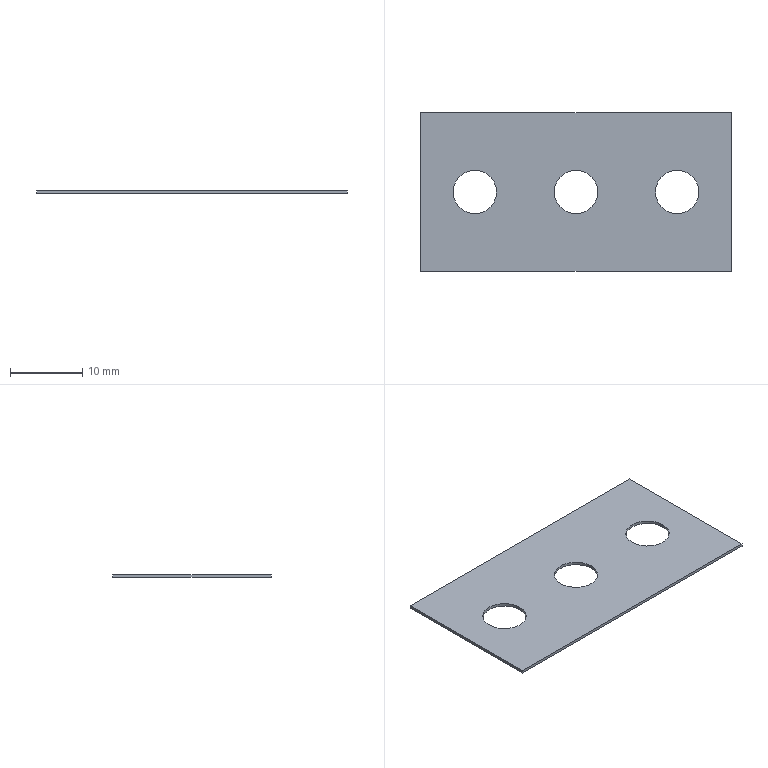Part | SolidWorks | features Extrusion 1, ICE 1 | 1 solid | 12 faces | box 43 x 22 x 0.4 mm | volume 344.471 mm3 | cylinder 6 | plane 6 | commonest cylinder face diameters 6 x6
STEP:
#1=CARTESIAN_POINT('',(11.,0.,0.));
#2=VERTEX_POINT('',#1);
#3=CARTESIAN_POINT('',(17.,0.,0.));
#4=VERTEX_POINT('',#3);
#5=CARTESIAN_POINT('',(14.,0.,0.));
#6=DIRECTION('',(0.,0.,1.));
#7=DIRECTION('',(1.,0.,0.));
#8=AXIS2_PLACEMENT_3D('',#5,#6,#7);
#9=CIRCLE('',#8,3.);
#10=EDGE_CURVE('',#2,#4,#9,.T.);
#11=ORIENTED_EDGE('',*,*,#10,.F.);
#12=CARTESIAN_POINT('',(11.,0.,0.4));
#13=VERTEX_POINT('',#12);
#14=CARTESIAN_POINT('',(11.,0.,0.));
#15=DIRECTION('',(0.,0.,1.));
#16=VECTOR('',#15,1000.);
#17=LINE('',#14,#16);
#18=EDGE_CURVE('',#2,#13,#17,.T.);
#19=ORIENTED_EDGE('',*,*,#18,.T.);
#20=CARTESIAN_POINT('',(17.,0.,0.4));
#21=VERTEX_POINT('',#20);
#22=CARTESIAN_POINT('',(14.,0.,0.4));
#23=DIRECTION('',(0.,0.,1.));
#24=DIRECTION('',(1.,0.,0.));
#25=AXIS2_PLACEMENT_3D('',#22,#23,#24);
#26=CIRCLE('',#25,3.);
#27=EDGE_CURVE('',#13,#21,#26,.T.);
#28=ORIENTED_EDGE('',*,*,#27,.T.);
#29=CARTESIAN_POINT('',(17.,0.,0.));
#30=DIRECTION('',(0.,0.,1.));
#31=VECTOR('',#30,1000.);
#32=LINE('',#29,#31);
#33=EDGE_CURVE('',#4,#21,#32,.T.);
#34=ORIENTED_EDGE('',*,*,#33,.F.);
#35=EDGE_LOOP('',(#11,#19,#28,#34));
#36=FACE_OUTER_BOUND('',#35,.T.);
#37=CARTESIAN_POINT('',(14.,0.,0.));
#38=DIRECTION('',(0.,0.,1.));
#39=DIRECTION('',(1.,0.,0.));
#40=AXIS2_PLACEMENT_3D('',#37,#38,#39);
#41=CYLINDRICAL_SURFACE('',#40,3.);
#42=ADVANCED_FACE('',(#36),#41,.F.);
#43=CARTESIAN_POINT('',(-17.,0.,0.));
#44=VERTEX_POINT('',#43);
#45=CARTESIAN_POINT('',(-11.,0.,0.));
#46=VERTEX_POINT('',#45);
#47=CARTESIAN_POINT('',(-14.,0.,0.));
#48=DIRECTION('',(0.,0.,1.));
#49=DIRECTION('',(1.,0.,0.));
#50=AXIS2_PLACEMENT_3D('',#47,#48,#49);
#51=CIRCLE('',#50,3.);
#52=EDGE_CURVE('',#44,#46,#51,.T.);
#53=ORIENTED_EDGE('',*,*,#52,.F.);
#54=CARTESIAN_POINT('',(-17.,0.,0.4));
#55=VERTEX_POINT('',#54);
#56=CARTESIAN_POINT('',(-17.,0.,0.));
#57=DIRECTION('',(0.,0.,1.));
#58=VECTOR('',#57,1000.);
#59=LINE('',#56,#58);
#60=EDGE_CURVE('',#44,#55,#59,.T.);
#61=ORIENTED_EDGE('',*,*,#60,.T.);
#62=CARTESIAN_POINT('',(-11.,0.,0.4));
#63=VERTEX_POINT('',#62);
#64=CARTESIAN_POINT('',(-14.,0.,0.4));
#65=DIRECTION('',(0.,0.,1.));
#66=DIRECTION('',(1.,0.,0.));
#67=AXIS2_PLACEMENT_3D('',#64,#65,#66);
#68=CIRCLE('',#67,3.);
#69=EDGE_CURVE('',#55,#63,#68,.T.);
#70=ORIENTED_EDGE('',*,*,#69,.T.);
#71=CARTESIAN_POINT('',(-11.,0.,0.));
#72=DIRECTION('',(0.,0.,1.));
#73=VECTOR('',#72,1000.);
#74=LINE('',#71,#73);
#75=EDGE_CURVE('',#46,#63,#74,.T.);
#76=ORIENTED_EDGE('',*,*,#75,.F.);
#77=EDGE_LOOP('',(#53,#61,#70,#76));
#78=FACE_OUTER_BOUND('',#77,.T.);
#79=CARTESIAN_POINT('',(-14.,0.,0.));
#80=DIRECTION('',(0.,0.,1.));
#81=DIRECTION('',(1.,0.,0.));
#82=AXIS2_PLACEMENT_3D('',#79,#80,#81);
#83=CYLINDRICAL_SURFACE('',#82,3.);
#84=ADVANCED_FACE('',(#78),#83,.F.);
#85=CARTESIAN_POINT('',(-3.,0.,0.));
#86=VERTEX_POINT('',#85);
#87=CARTESIAN_POINT('',(3.,0.,0.));
#88=VERTEX_POINT('',#87);
#89=CARTESIAN_POINT('',(0.,0.,0.));
#90=DIRECTION('',(0.,0.,1.));
#91=DIRECTION('',(1.,0.,0.));
#92=AXIS2_PLACEMENT_3D('',#89,#90,#91);
#93=CIRCLE('',#92,3.);
#94=EDGE_CURVE('',#86,#88,#93,.T.);
#95=ORIENTED_EDGE('',*,*,#94,.F.);
#96=CARTESIAN_POINT('',(-3.,0.,0.4));
#97=VERTEX_POINT('',#96);
#98=CARTESIAN_POINT('',(-3.,0.,0.));
#99=DIRECTION('',(0.,0.,1.));
#100=VECTOR('',#99,1000.);
#101=LINE('',#98,#100);
#102=EDGE_CURVE('',#86,#97,#101,.T.);
#103=ORIENTED_EDGE('',*,*,#102,.T.);
#104=CARTESIAN_POINT('',(3.,0.,0.4));
#105=VERTEX_POINT('',#104);
#106=CARTESIAN_POINT('',(0.,0.,0.4));
#107=DIRECTION('',(0.,0.,1.));
#108=DIRECTION('',(1.,0.,0.));
#109=AXIS2_PLACEMENT_3D('',#106,#107,#108);
#110=CIRCLE('',#109,3.);
#111=EDGE_CURVE('',#97,#105,#110,.T.);
#112=ORIENTED_EDGE('',*,*,#111,.T.);
#113=CARTESIAN_POINT('',(3.,0.,0.));
#114=DIRECTION('',(0.,0.,1.));
#115=VECTOR('',#114,1000.);
#116=LINE('',#113,#115);
#117=EDGE_CURVE('',#88,#105,#116,.T.);
#118=ORIENTED_EDGE('',*,*,#117,.F.);
#119=EDGE_LOOP('',(#95,#103,#112,#118));
#120=FACE_OUTER_BOUND('',#119,.T.);
#121=CARTESIAN_POINT('',(0.,0.,0.));
#122=DIRECTION('',(0.,0.,1.));
#123=DIRECTION('',(1.,0.,0.));
#124=AXIS2_PLACEMENT_3D('',#121,#122,#123);
#125=CYLINDRICAL_SURFACE('',#124,3.);
#126=ADVANCED_FACE('',(#120),#125,.F.);
#127=CARTESIAN_POINT('',(21.5,-11.,0.));
#128=VERTEX_POINT('',#127);
#129=CARTESIAN_POINT('',(21.5,11.,0.));
#130=VERTEX_POINT('',#129);
#131=CARTESIAN_POINT('',(21.5,-11.,0.));
#132=DIRECTION('',(0.,1.,0.));
#133=VECTOR('',#132,1000.);
#134=LINE('',#131,#133);
#135=EDGE_CURVE('',#128,#130,#134,.T.);
#136=ORIENTED_EDGE('',*,*,#135,.T.);
#137=CARTESIAN_POINT('',(21.5,11.,0.4));
#138=VERTEX_POINT('',#137);
#139=CARTESIAN_POINT('',(21.5,11.,0.4));
#140=DIRECTION('',(0.,0.,-1.));
#141=VECTOR('',#140,1000.);
#142=LINE('',#139,#141);
#143=EDGE_CURVE('',#138,#130,#142,.T.);
#144=ORIENTED_EDGE('',*,*,#143,.F.);
#145=CARTESIAN_POINT('',(21.5,-11.,0.4));
#146=VERTEX_POINT('',#145);
#147=CARTESIAN_POINT('',(21.5,-11.,0.4));
#148=DIRECTION('',(0.,1.,0.));
#149=VECTOR('',#148,1000.);
#150=LINE('',#147,#149);
#151=EDGE_CURVE('',#146,#138,#150,.T.);
#152=ORIENTED_EDGE('',*,*,#151,.F.);
#153=CARTESIAN_POINT('',(21.5,-11.,0.4));
#154=DIRECTION('',(0.,0.,-1.));
#155=VECTOR('',#154,1000.);
#156=LINE('',#153,#155);
#157=EDGE_CURVE('',#146,#128,#156,.T.);
#158=ORIENTED_EDGE('',*,*,#157,.T.);
#159=EDGE_LOOP('',(#136,#144,#152,#158));
#160=FACE_OUTER_BOUND('',#159,.T.);
#161=CARTESIAN_POINT('',(21.5,-11.,0.4));
#162=DIRECTION('',(-1.,0.,0.));
#163=DIRECTION('',(0.,0.,1.));
#164=AXIS2_PLACEMENT_3D('',#161,#162,#163);
#165=PLANE('',#164);
#166=ADVANCED_FACE('',(#160),#165,.F.);
#167=CARTESIAN_POINT('',(-21.5,11.,0.));
#168=VERTEX_POINT('',#167);
#169=CARTESIAN_POINT('',(-21.5,11.,0.));
#170=DIRECTION('',(-1.,0.,0.));
#171=VECTOR('',#170,1000.);
#172=LINE('',#169,#171);
#173=EDGE_CURVE('',#130,#168,#172,.T.);
#174=ORIENTED_EDGE('',*,*,#173,.T.);
#175=CARTESIAN_POINT('',(-21.5,11.,0.4));
#176=VERTEX_POINT('',#175);
#177=CARTESIAN_POINT('',(-21.5,11.,0.4));
#178=DIRECTION('',(0.,0.,-1.));
#179=VECTOR('',#178,1000.);
#180=LINE('',#177,#179);
#181=EDGE_CURVE('',#176,#168,#180,.T.);
#182=ORIENTED_EDGE('',*,*,#181,.F.);
#183=CARTESIAN_POINT('',(-21.5,11.,0.4));
#184=DIRECTION('',(-1.,0.,0.));
#185=VECTOR('',#184,1000.);
#186=LINE('',#183,#185);
#187=EDGE_CURVE('',#138,#176,#186,.T.);
#188=ORIENTED_EDGE('',*,*,#187,.F.);
#189=ORIENTED_EDGE('',*,*,#143,.T.);
#190=EDGE_LOOP('',(#174,#182,#188,#189));
#191=FACE_OUTER_BOUND('',#190,.T.);
#192=CARTESIAN_POINT('',(-21.5,11.,0.4));
#193=DIRECTION('',(0.,-1.,0.));
#194=DIRECTION('',(0.,0.,-1.));
#195=AXIS2_PLACEMENT_3D('',#192,#193,#194);
#196=PLANE('',#195);
#197=ADVANCED_FACE('',(#191),#196,.F.);
#198=CARTESIAN_POINT('',(-21.5,-11.,0.));
#199=VERTEX_POINT('',#198);
#200=CARTESIAN_POINT('',(-21.5,-11.,0.));
#201=DIRECTION('',(0.,-1.,0.));
#202=VECTOR('',#201,1000.);
#203=LINE('',#200,#202);
#204=EDGE_CURVE('',#168,#199,#203,.T.);
#205=ORIENTED_EDGE('',*,*,#204,.T.);
#206=CARTESIAN_POINT('',(-21.5,-11.,0.4));
#207=VERTEX_POINT('',#206);
#208=CARTESIAN_POINT('',(-21.5,-11.,0.4));
#209=DIRECTION('',(0.,0.,-1.));
#210=VECTOR('',#209,1000.);
#211=LINE('',#208,#210);
#212=EDGE_CURVE('',#207,#199,#211,.T.);
#213=ORIENTED_EDGE('',*,*,#212,.F.);
#214=CARTESIAN_POINT('',(-21.5,-11.,0.4));
#215=DIRECTION('',(0.,-1.,0.));
#216=VECTOR('',#215,1000.);
#217=LINE('',#214,#216);
#218=EDGE_CURVE('',#176,#207,#217,.T.);
#219=ORIENTED_EDGE('',*,*,#218,.F.);
#220=ORIENTED_EDGE('',*,*,#181,.T.);
#221=EDGE_LOOP('',(#205,#213,#219,#220));
#222=FACE_OUTER_BOUND('',#221,.T.);
#223=CARTESIAN_POINT('',(-21.5,-11.,0.4));
#224=DIRECTION('',(1.,0.,0.));
#225=DIRECTION('',(0.,0.,-1.));
#226=AXIS2_PLACEMENT_3D('',#223,#224,#225);
#227=PLANE('',#226);
#228=ADVANCED_FACE('',(#222),#227,.F.);
#229=CARTESIAN_POINT('',(-21.5,-11.,0.));
#230=DIRECTION('',(1.,0.,0.));
#231=VECTOR('',#230,1000.);
#232=LINE('',#229,#231);
#233=EDGE_CURVE('',#199,#128,#232,.T.);
#234=ORIENTED_EDGE('',*,*,#233,.T.);
#235=ORIENTED_EDGE('',*,*,#157,.F.);
#236=CARTESIAN_POINT('',(-21.5,-11.,0.4));
#237=DIRECTION('',(1.,0.,0.));
#238=VECTOR('',#237,1000.);
#239=LINE('',#236,#238);
#240=EDGE_CURVE('',#207,#146,#239,.T.);
#241=ORIENTED_EDGE('',*,*,#240,.F.);
#242=ORIENTED_EDGE('',*,*,#212,.T.);
#243=EDGE_LOOP('',(#234,#235,#241,#242));
#244=FACE_OUTER_BOUND('',#243,.T.);
#245=CARTESIAN_POINT('',(-21.5,-11.,0.4));
#246=DIRECTION('',(0.,1.,0.));
#247=DIRECTION('',(0.,0.,1.));
#248=AXIS2_PLACEMENT_3D('',#245,#246,#247);
#249=PLANE('',#248);
#250=ADVANCED_FACE('',(#244),#249,.F.);
#251=CARTESIAN_POINT('',(14.,0.,0.4));
#252=DIRECTION('',(0.,0.,1.));
#253=DIRECTION('',(1.,0.,0.));
#254=AXIS2_PLACEMENT_3D('',#251,#252,#253);
#255=CIRCLE('',#254,3.);
#256=EDGE_CURVE('',#21,#13,#255,.T.);
#257=ORIENTED_EDGE('',*,*,#256,.F.);
#258=ORIENTED_EDGE('',*,*,#27,.F.);
#259=EDGE_LOOP('',(#257,#258));
#260=FACE_BOUND('',#259,.T.);
#261=CARTESIAN_POINT('',(-14.,0.,0.4));
#262=DIRECTION('',(0.,0.,1.));
#263=DIRECTION('',(1.,0.,0.));
#264=AXIS2_PLACEMENT_3D('',#261,#262,#263);
#265=CIRCLE('',#264,3.);
#266=EDGE_CURVE('',#63,#55,#265,.T.);
#267=ORIENTED_EDGE('',*,*,#266,.F.);
#268=ORIENTED_EDGE('',*,*,#69,.F.);
#269=EDGE_LOOP('',(#267,#268));
#270=FACE_BOUND('',#269,.T.);
#271=CARTESIAN_POINT('',(0.,0.,0.4));
#272=DIRECTION('',(0.,0.,1.));
#273=DIRECTION('',(1.,0.,0.));
#274=AXIS2_PLACEMENT_3D('',#271,#272,#273);
#275=CIRCLE('',#274,3.);
#276=EDGE_CURVE('',#105,#97,#275,.T.);
#277=ORIENTED_EDGE('',*,*,#276,.F.);
#278=ORIENTED_EDGE('',*,*,#111,.F.);
#279=EDGE_LOOP('',(#277,#278));
#280=FACE_BOUND('',#279,.T.);
#281=ORIENTED_EDGE('',*,*,#151,.T.);
#282=ORIENTED_EDGE('',*,*,#187,.T.);
#283=ORIENTED_EDGE('',*,*,#218,.T.);
#284=ORIENTED_EDGE('',*,*,#240,.T.);
#285=EDGE_LOOP('',(#281,#282,#283,#284));
#286=FACE_OUTER_BOUND('',#285,.T.);
#287=CARTESIAN_POINT('',(0.,0.,0.4));
#288=DIRECTION('',(0.,0.,-1.));
#289=DIRECTION('',(-1.,0.,0.));
#290=AXIS2_PLACEMENT_3D('',#287,#288,#289);
#291=PLANE('',#290);
#292=ADVANCED_FACE('',(#260,#270,#280,#286),#291,.F.);
#293=CARTESIAN_POINT('',(14.,0.,0.));
#294=DIRECTION('',(0.,0.,1.));
#295=DIRECTION('',(1.,0.,0.));
#296=AXIS2_PLACEMENT_3D('',#293,#294,#295);
#297=CIRCLE('',#296,3.);
#298=EDGE_CURVE('',#4,#2,#297,.T.);
#299=ORIENTED_EDGE('',*,*,#298,.T.);
#300=ORIENTED_EDGE('',*,*,#10,.T.);
#301=EDGE_LOOP('',(#299,#300));
#302=FACE_BOUND('',#301,.T.);
#303=CARTESIAN_POINT('',(-14.,0.,0.));
#304=DIRECTION('',(0.,0.,1.));
#305=DIRECTION('',(1.,0.,0.));
#306=AXIS2_PLACEMENT_3D('',#303,#304,#305);
#307=CIRCLE('',#306,3.);
#308=EDGE_CURVE('',#46,#44,#307,.T.);
#309=ORIENTED_EDGE('',*,*,#308,.T.);
#310=ORIENTED_EDGE('',*,*,#52,.T.);
#311=EDGE_LOOP('',(#309,#310));
#312=FACE_BOUND('',#311,.T.);
#313=CARTESIAN_POINT('',(0.,0.,0.));
#314=DIRECTION('',(0.,0.,1.));
#315=DIRECTION('',(1.,0.,0.));
#316=AXIS2_PLACEMENT_3D('',#313,#314,#315);
#317=CIRCLE('',#316,3.);
#318=EDGE_CURVE('',#88,#86,#317,.T.);
#319=ORIENTED_EDGE('',*,*,#318,.T.);
#320=ORIENTED_EDGE('',*,*,#94,.T.);
#321=EDGE_LOOP('',(#319,#320));
#322=FACE_BOUND('',#321,.T.);
#323=ORIENTED_EDGE('',*,*,#135,.F.);
#324=ORIENTED_EDGE('',*,*,#233,.F.);
#325=ORIENTED_EDGE('',*,*,#204,.F.);
#326=ORIENTED_EDGE('',*,*,#173,.F.);
#327=EDGE_LOOP('',(#323,#324,#325,#326));
#328=FACE_OUTER_BOUND('',#327,.T.);
#329=CARTESIAN_POINT('',(0.,0.,0.));
#330=DIRECTION('',(0.,0.,-1.));
#331=DIRECTION('',(-1.,0.,0.));
#332=AXIS2_PLACEMENT_3D('',#329,#330,#331);
#333=PLANE('',#332);
#334=ADVANCED_FACE('',(#302,#312,#322,#328),#333,.T.);
#335=ORIENTED_EDGE('',*,*,#102,.F.);
#336=ORIENTED_EDGE('',*,*,#318,.F.);
#337=ORIENTED_EDGE('',*,*,#117,.T.);
#338=ORIENTED_EDGE('',*,*,#276,.T.);
#339=EDGE_LOOP('',(#335,#336,#337,#338));
#340=FACE_OUTER_BOUND('',#339,.T.);
#341=CARTESIAN_POINT('',(0.,0.,0.));
#342=DIRECTION('',(0.,0.,1.));
#343=DIRECTION('',(1.,0.,0.));
#344=AXIS2_PLACEMENT_3D('',#341,#342,#343);
#345=CYLINDRICAL_SURFACE('',#344,3.);
#346=ADVANCED_FACE('',(#340),#345,.F.);
#347=ORIENTED_EDGE('',*,*,#60,.F.);
#348=ORIENTED_EDGE('',*,*,#308,.F.);
#349=ORIENTED_EDGE('',*,*,#75,.T.);
#350=ORIENTED_EDGE('',*,*,#266,.T.);
#351=EDGE_LOOP('',(#347,#348,#349,#350));
#352=FACE_OUTER_BOUND('',#351,.T.);
#353=CARTESIAN_POINT('',(-14.,0.,0.));
#354=DIRECTION('',(0.,0.,1.));
#355=DIRECTION('',(1.,0.,0.));
#356=AXIS2_PLACEMENT_3D('',#353,#354,#355);
#357=CYLINDRICAL_SURFACE('',#356,3.);
#358=ADVANCED_FACE('',(#352),#357,.F.);
#359=ORIENTED_EDGE('',*,*,#18,.F.);
#360=ORIENTED_EDGE('',*,*,#298,.F.);
#361=ORIENTED_EDGE('',*,*,#33,.T.);
#362=ORIENTED_EDGE('',*,*,#256,.T.);
#363=EDGE_LOOP('',(#359,#360,#361,#362));
#364=FACE_OUTER_BOUND('',#363,.T.);
#365=CARTESIAN_POINT('',(14.,0.,0.));
#366=DIRECTION('',(0.,0.,1.));
#367=DIRECTION('',(1.,0.,0.));
#368=AXIS2_PLACEMENT_3D('',#365,#366,#367);
#369=CYLINDRICAL_SURFACE('',#368,3.);
#370=ADVANCED_FACE('',(#364),#369,.F.);
#371=CLOSED_SHELL('',(#42,#84,#126,#166,#197,#228,#250,#292,#334,#346,#358,#370));
#372=MANIFOLD_SOLID_BREP('',#371);
#373=CARTESIAN_POINT('',(0.,0.,0.));
#374=DIRECTION('',(0.,0.,1.));
#375=DIRECTION('',(1.,0.,0.));
#376=AXIS2_PLACEMENT_3D('',#373,#374,#375);
#377=(LENGTH_UNIT()NAMED_UNIT(*)SI_UNIT(.MILLI.,.METRE.));
#378=UNCERTAINTY_MEASURE_WITH_UNIT(LENGTH_MEASURE(0.00001),#377,'','');
#379=(NAMED_UNIT(*)PLANE_ANGLE_UNIT()SI_UNIT($,.RADIAN.));
#380=(NAMED_UNIT(*)SI_UNIT($,.STERADIAN.)SOLID_ANGLE_UNIT());
#381=(GEOMETRIC_REPRESENTATION_CONTEXT(3)GLOBAL_UNCERTAINTY_ASSIGNED_CONTEXT((#378))GLOBAL_UNIT_ASSIGNED_CONTEXT((#377,#379,#380))REPRESENTATION_CONTEXT('',''));
#382=ADVANCED_BREP_SHAPE_REPRESENTATION('',(#372,#376),#381);